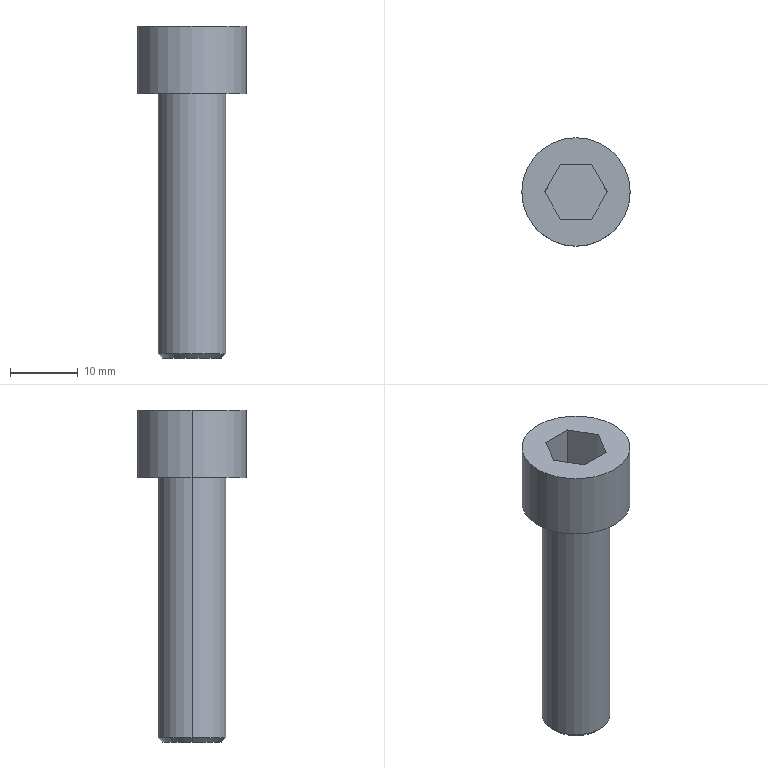Part | Creo | 1 solid | 16 faces | box 16 x 16 x 49 mm | volume 4702 mm3 | plane 10 | cylinder 4 | cone 2 | commonest cylinder face diameters 10 x2 16 x2
STEP:
#1=CARTESIAN_POINT('',(0.,0.,0.));
#2=DIRECTION('',(0.,0.,1.));
#3=DIRECTION('',(1.,0.,0.));
#4=AXIS2_PLACEMENT_3D('',#1,#2,#3);
#5=CARTESIAN_POINT('',(-234.899,34.764,-141.184));
#6=VERTEX_POINT('',#5);
#7=CARTESIAN_POINT('',(-224.899,34.764,-141.184));
#8=VERTEX_POINT('',#7);
#9=CARTESIAN_POINT('',(-229.899,34.764,-141.184));
#10=DIRECTION('',(0.,0.,-1.));
#11=DIRECTION('',(-1.,0.,0.));
#12=AXIS2_PLACEMENT_3D('',#9,#10,#11);
#13=CIRCLE('',#12,5.);
#14=EDGE_CURVE('',#6,#8,#13,.T.);
#15=ORIENTED_EDGE('',*,*,#14,.T.);
#16=CARTESIAN_POINT('',(-224.899,34.764,-102.793));
#17=VERTEX_POINT('',#16);
#18=CARTESIAN_POINT('',(-224.899,34.764,-102.793));
#19=DIRECTION('',(0.,0.,-1.));
#20=VECTOR('',#19,38.391);
#21=LINE('',#18,#20);
#22=EDGE_CURVE('',#17,#8,#21,.T.);
#23=ORIENTED_EDGE('',*,*,#22,.F.);
#24=CARTESIAN_POINT('',(-234.899,34.764,-102.793));
#25=VERTEX_POINT('',#24);
#26=CARTESIAN_POINT('',(-229.899,34.764,-102.793));
#27=DIRECTION('',(0.,0.,1.));
#28=DIRECTION('',(1.,0.,0.));
#29=AXIS2_PLACEMENT_3D('',#26,#27,#28);
#30=CIRCLE('',#29,5.);
#31=EDGE_CURVE('',#17,#25,#30,.T.);
#32=ORIENTED_EDGE('',*,*,#31,.T.);
#33=CARTESIAN_POINT('',(-234.899,34.764,-102.793));
#34=DIRECTION('',(0.,0.,-1.));
#35=VECTOR('',#34,38.391);
#36=LINE('',#33,#35);
#37=EDGE_CURVE('',#25,#6,#36,.T.);
#38=ORIENTED_EDGE('',*,*,#37,.T.);
#39=EDGE_LOOP('',(#15,#23,#32,#38));
#40=FACE_OUTER_BOUND('',#39,.F.);
#41=CARTESIAN_POINT('',(-229.899,34.764,-102.793));
#42=DIRECTION('',(0.,0.,-1.));
#43=DIRECTION('',(-1.,0.,0.));
#44=AXIS2_PLACEMENT_3D('',#41,#42,#43);
#45=CYLINDRICAL_SURFACE('',#44,5.);
#46=ADVANCED_FACE('',(#40),#45,.T.);
#47=CARTESIAN_POINT('',(-234.29,34.764,-141.793));
#48=VERTEX_POINT('',#47);
#49=CARTESIAN_POINT('',(-225.508,34.764,-141.793));
#50=VERTEX_POINT('',#49);
#51=CARTESIAN_POINT('',(-229.899,34.764,-141.793));
#52=DIRECTION('',(0.,0.,-1.));
#53=DIRECTION('',(-1.,0.,0.));
#54=AXIS2_PLACEMENT_3D('',#51,#52,#53);
#55=CIRCLE('',#54,4.391);
#56=EDGE_CURVE('',#48,#50,#55,.T.);
#57=ORIENTED_EDGE('',*,*,#56,.T.);
#58=CARTESIAN_POINT('',(-225.508,34.764,-141.793));
#59=DIRECTION('',(0.7071,0.,0.7071));
#60=VECTOR('',#59,0.8611);
#61=LINE('',#58,#60);
#62=EDGE_CURVE('',#50,#8,#61,.T.);
#63=ORIENTED_EDGE('',*,*,#62,.T.);
#64=ORIENTED_EDGE('',*,*,#14,.F.);
#65=CARTESIAN_POINT('',(-234.29,34.764,-141.793));
#66=DIRECTION('',(-0.7071,0.,0.7071));
#67=VECTOR('',#66,0.8611);
#68=LINE('',#65,#67);
#69=EDGE_CURVE('',#48,#6,#68,.T.);
#70=ORIENTED_EDGE('',*,*,#69,.F.);
#71=EDGE_LOOP('',(#57,#63,#64,#70));
#72=FACE_OUTER_BOUND('',#71,.F.);
#73=CARTESIAN_POINT('',(-229.899,34.764,-141.489));
#74=DIRECTION('',(0.,0.,1.));
#75=DIRECTION('',(1.,0.,0.));
#76=AXIS2_PLACEMENT_3D('',#73,#74,#75);
#77=CONICAL_SURFACE('',#76,4.696,45.);
#78=ADVANCED_FACE('',(#72),#77,.T.);
#79=CARTESIAN_POINT('',(-229.899,34.764,-141.793));
#80=DIRECTION('',(0.,0.,-1.));
#81=DIRECTION('',(1.,0.,0.));
#82=AXIS2_PLACEMENT_3D('',#79,#80,#81);
#83=CIRCLE('',#82,4.391);
#84=EDGE_CURVE('',#50,#48,#83,.T.);
#85=ORIENTED_EDGE('',*,*,#84,.F.);
#86=ORIENTED_EDGE('',*,*,#56,.F.);
#87=EDGE_LOOP('',(#85,#86));
#88=FACE_OUTER_BOUND('',#87,.F.);
#89=CARTESIAN_POINT('',(-229.899,34.764,-141.793));
#90=DIRECTION('',(0.,0.,1.));
#91=DIRECTION('',(1.,0.,0.));
#92=AXIS2_PLACEMENT_3D('',#89,#90,#91);
#93=PLANE('',#92);
#94=ADVANCED_FACE('',(#88),#93,.F.);
#95=ORIENTED_EDGE('',*,*,#84,.T.);
#96=ORIENTED_EDGE('',*,*,#69,.T.);
#97=CARTESIAN_POINT('',(-229.899,34.764,-141.184));
#98=DIRECTION('',(0.,0.,-1.));
#99=DIRECTION('',(1.,0.,0.));
#100=AXIS2_PLACEMENT_3D('',#97,#98,#99);
#101=CIRCLE('',#100,5.);
#102=EDGE_CURVE('',#8,#6,#101,.T.);
#103=ORIENTED_EDGE('',*,*,#102,.F.);
#104=ORIENTED_EDGE('',*,*,#62,.F.);
#105=EDGE_LOOP('',(#95,#96,#103,#104));
#106=FACE_OUTER_BOUND('',#105,.F.);
#107=CARTESIAN_POINT('',(-229.899,34.764,-141.489));
#108=DIRECTION('',(0.,0.,1.));
#109=DIRECTION('',(1.,0.,0.));
#110=AXIS2_PLACEMENT_3D('',#107,#108,#109);
#111=CONICAL_SURFACE('',#110,4.696,45.);
#112=ADVANCED_FACE('',(#106),#111,.T.);
#113=ORIENTED_EDGE('',*,*,#102,.T.);
#114=ORIENTED_EDGE('',*,*,#37,.F.);
#115=CARTESIAN_POINT('',(-229.899,34.764,-102.793));
#116=DIRECTION('',(0.,0.,1.));
#117=DIRECTION('',(-1.,0.,0.));
#118=AXIS2_PLACEMENT_3D('',#115,#116,#117);
#119=CIRCLE('',#118,5.);
#120=EDGE_CURVE('',#25,#17,#119,.T.);
#121=ORIENTED_EDGE('',*,*,#120,.T.);
#122=ORIENTED_EDGE('',*,*,#22,.T.);
#123=EDGE_LOOP('',(#113,#114,#121,#122));
#124=FACE_OUTER_BOUND('',#123,.F.);
#125=CARTESIAN_POINT('',(-229.899,34.764,-102.793));
#126=DIRECTION('',(0.,0.,-1.));
#127=DIRECTION('',(-1.,0.,0.));
#128=AXIS2_PLACEMENT_3D('',#125,#126,#127);
#129=CYLINDRICAL_SURFACE('',#128,5.);
#130=ADVANCED_FACE('',(#124),#129,.T.);
#131=CARTESIAN_POINT('',(-221.899,34.764,-102.793));
#132=VERTEX_POINT('',#131);
#133=CARTESIAN_POINT('',(-237.899,34.764,-102.793));
#134=VERTEX_POINT('',#133);
#135=CARTESIAN_POINT('',(-229.899,34.764,-102.793));
#136=DIRECTION('',(0.,0.,-1.));
#137=DIRECTION('',(1.,0.,0.));
#138=AXIS2_PLACEMENT_3D('',#135,#136,#137);
#139=CIRCLE('',#138,8.);
#140=EDGE_CURVE('',#132,#134,#139,.T.);
#141=ORIENTED_EDGE('',*,*,#140,.F.);
#142=CARTESIAN_POINT('',(-229.899,34.764,-102.793));
#143=DIRECTION('',(0.,0.,-1.));
#144=DIRECTION('',(-1.,0.,0.));
#145=AXIS2_PLACEMENT_3D('',#142,#143,#144);
#146=CIRCLE('',#145,8.);
#147=EDGE_CURVE('',#134,#132,#146,.T.);
#148=ORIENTED_EDGE('',*,*,#147,.F.);
#149=EDGE_LOOP('',(#141,#148));
#150=FACE_OUTER_BOUND('',#149,.F.);
#151=ORIENTED_EDGE('',*,*,#31,.F.);
#152=ORIENTED_EDGE('',*,*,#120,.F.);
#153=EDGE_LOOP('',(#151,#152));
#154=FACE_BOUND('',#153,.F.);
#155=CARTESIAN_POINT('',(-229.899,34.764,-102.793));
#156=DIRECTION('',(0.,0.,-1.));
#157=DIRECTION('',(-1.,0.,0.));
#158=AXIS2_PLACEMENT_3D('',#155,#156,#157);
#159=PLANE('',#158);
#160=ADVANCED_FACE('',(#150,#154),#159,.T.);
#161=CARTESIAN_POINT('',(-237.899,34.764,-92.793));
#162=VERTEX_POINT('',#161);
#163=CARTESIAN_POINT('',(-221.899,34.764,-92.793));
#164=VERTEX_POINT('',#163);
#165=CARTESIAN_POINT('',(-229.899,34.764,-92.793));
#166=DIRECTION('',(0.,0.,1.));
#167=DIRECTION('',(-1.,0.,0.));
#168=AXIS2_PLACEMENT_3D('',#165,#166,#167);
#169=CIRCLE('',#168,8.);
#170=EDGE_CURVE('',#162,#164,#169,.T.);
#171=ORIENTED_EDGE('',*,*,#170,.T.);
#172=CARTESIAN_POINT('',(-221.899,34.764,-102.793));
#173=DIRECTION('',(0.,0.,1.));
#174=VECTOR('',#173,10.);
#175=LINE('',#172,#174);
#176=EDGE_CURVE('',#132,#164,#175,.T.);
#177=ORIENTED_EDGE('',*,*,#176,.F.);
#178=ORIENTED_EDGE('',*,*,#140,.T.);
#179=CARTESIAN_POINT('',(-237.899,34.764,-102.793));
#180=DIRECTION('',(0.,0.,1.));
#181=VECTOR('',#180,10.);
#182=LINE('',#179,#181);
#183=EDGE_CURVE('',#134,#162,#182,.T.);
#184=ORIENTED_EDGE('',*,*,#183,.T.);
#185=EDGE_LOOP('',(#171,#177,#178,#184));
#186=FACE_OUTER_BOUND('',#185,.F.);
#187=CARTESIAN_POINT('',(-229.899,34.764,-102.793));
#188=DIRECTION('',(0.,0.,1.));
#189=DIRECTION('',(1.,0.,0.));
#190=AXIS2_PLACEMENT_3D('',#187,#188,#189);
#191=CYLINDRICAL_SURFACE('',#190,8.);
#192=ADVANCED_FACE('',(#186),#191,.T.);
#193=CARTESIAN_POINT('',(-229.899,34.764,-92.793));
#194=DIRECTION('',(0.,0.,1.));
#195=DIRECTION('',(1.,0.,0.));
#196=AXIS2_PLACEMENT_3D('',#193,#194,#195);
#197=CIRCLE('',#196,8.);
#198=EDGE_CURVE('',#164,#162,#197,.T.);
#199=ORIENTED_EDGE('',*,*,#198,.F.);
#200=ORIENTED_EDGE('',*,*,#170,.F.);
#201=EDGE_LOOP('',(#199,#200));
#202=FACE_OUTER_BOUND('',#201,.F.);
#203=CARTESIAN_POINT('',(-227.59,30.764,-92.793));
#204=VERTEX_POINT('',#203);
#205=CARTESIAN_POINT('',(-232.209,30.764,-92.793));
#206=VERTEX_POINT('',#205);
#207=CARTESIAN_POINT('',(-227.59,30.764,-92.793));
#208=DIRECTION('',(-1.,0.,0.));
#209=VECTOR('',#208,4.619);
#210=LINE('',#207,#209);
#211=EDGE_CURVE('',#204,#206,#210,.T.);
#212=ORIENTED_EDGE('',*,*,#211,.F.);
#213=CARTESIAN_POINT('',(-225.28,34.764,-92.793));
#214=VERTEX_POINT('',#213);
#215=CARTESIAN_POINT('',(-225.28,34.764,-92.793));
#216=DIRECTION('',(-0.5,-0.866,0.));
#217=VECTOR('',#216,4.619);
#218=LINE('',#215,#217);
#219=EDGE_CURVE('',#214,#204,#218,.T.);
#220=ORIENTED_EDGE('',*,*,#219,.F.);
#221=CARTESIAN_POINT('',(-227.59,38.764,-92.793));
#222=VERTEX_POINT('',#221);
#223=CARTESIAN_POINT('',(-227.59,38.764,-92.793));
#224=DIRECTION('',(0.5,-0.866,0.));
#225=VECTOR('',#224,4.619);
#226=LINE('',#223,#225);
#227=EDGE_CURVE('',#222,#214,#226,.T.);
#228=ORIENTED_EDGE('',*,*,#227,.F.);
#229=CARTESIAN_POINT('',(-232.209,38.764,-92.793));
#230=VERTEX_POINT('',#229);
#231=CARTESIAN_POINT('',(-232.209,38.764,-92.793));
#232=DIRECTION('',(1.,0.,0.));
#233=VECTOR('',#232,4.619);
#234=LINE('',#231,#233);
#235=EDGE_CURVE('',#230,#222,#234,.T.);
#236=ORIENTED_EDGE('',*,*,#235,.F.);
#237=CARTESIAN_POINT('',(-234.518,34.764,-92.793));
#238=VERTEX_POINT('',#237);
#239=CARTESIAN_POINT('',(-234.518,34.764,-92.793));
#240=DIRECTION('',(0.5,0.866,0.));
#241=VECTOR('',#240,4.619);
#242=LINE('',#239,#241);
#243=EDGE_CURVE('',#238,#230,#242,.T.);
#244=ORIENTED_EDGE('',*,*,#243,.F.);
#245=CARTESIAN_POINT('',(-232.209,30.764,-92.793));
#246=DIRECTION('',(-0.5,0.866,0.));
#247=VECTOR('',#246,4.619);
#248=LINE('',#245,#247);
#249=EDGE_CURVE('',#206,#238,#248,.T.);
#250=ORIENTED_EDGE('',*,*,#249,.F.);
#251=EDGE_LOOP('',(#212,#220,#228,#236,#244,#250));
#252=FACE_BOUND('',#251,.F.);
#253=CARTESIAN_POINT('',(-229.899,34.764,-92.793));
#254=DIRECTION('',(0.,0.,1.));
#255=DIRECTION('',(1.,0.,0.));
#256=AXIS2_PLACEMENT_3D('',#253,#254,#255);
#257=PLANE('',#256);
#258=ADVANCED_FACE('',(#202,#252),#257,.T.);
#259=ORIENTED_EDGE('',*,*,#211,.T.);
#260=CARTESIAN_POINT('',(-232.209,30.764,-99.393));
#261=VERTEX_POINT('',#260);
#262=CARTESIAN_POINT('',(-232.209,30.764,-92.793));
#263=DIRECTION('',(0.,0.,-1.));
#264=VECTOR('',#263,6.6);
#265=LINE('',#262,#264);
#266=EDGE_CURVE('',#206,#261,#265,.T.);
#267=ORIENTED_EDGE('',*,*,#266,.T.);
#268=CARTESIAN_POINT('',(-227.59,30.764,-99.393));
#269=VERTEX_POINT('',#268);
#270=CARTESIAN_POINT('',(-227.59,30.764,-99.393));
#271=DIRECTION('',(-1.,0.,0.));
#272=VECTOR('',#271,4.619);
#273=LINE('',#270,#272);
#274=EDGE_CURVE('',#269,#261,#273,.T.);
#275=ORIENTED_EDGE('',*,*,#274,.F.);
#276=CARTESIAN_POINT('',(-227.59,30.764,-92.793));
#277=DIRECTION('',(0.,0.,-1.));
#278=VECTOR('',#277,6.6);
#279=LINE('',#276,#278);
#280=EDGE_CURVE('',#204,#269,#279,.T.);
#281=ORIENTED_EDGE('',*,*,#280,.F.);
#282=EDGE_LOOP('',(#259,#267,#275,#281));
#283=FACE_OUTER_BOUND('',#282,.F.);
#284=CARTESIAN_POINT('',(-232.209,30.764,-99.393));
#285=DIRECTION('',(0.,-1.,0.));
#286=DIRECTION('',(0.,0.,-1.));
#287=AXIS2_PLACEMENT_3D('',#284,#285,#286);
#288=PLANE('',#287);
#289=ADVANCED_FACE('',(#283),#288,.F.);
#290=ORIENTED_EDGE('',*,*,#249,.T.);
#291=CARTESIAN_POINT('',(-234.518,34.764,-99.393));
#292=VERTEX_POINT('',#291);
#293=CARTESIAN_POINT('',(-234.518,34.764,-92.793));
#294=DIRECTION('',(0.,0.,-1.));
#295=VECTOR('',#294,6.6);
#296=LINE('',#293,#295);
#297=EDGE_CURVE('',#238,#292,#296,.T.);
#298=ORIENTED_EDGE('',*,*,#297,.T.);
#299=CARTESIAN_POINT('',(-234.518,34.764,-99.393));
#300=DIRECTION('',(0.5,-0.866,0.));
#301=VECTOR('',#300,4.619);
#302=LINE('',#299,#301);
#303=EDGE_CURVE('',#292,#261,#302,.T.);
#304=ORIENTED_EDGE('',*,*,#303,.T.);
#305=ORIENTED_EDGE('',*,*,#266,.F.);
#306=EDGE_LOOP('',(#290,#298,#304,#305));
#307=FACE_OUTER_BOUND('',#306,.F.);
#308=CARTESIAN_POINT('',(-234.518,34.764,-99.393));
#309=DIRECTION('',(-0.866,-0.5,0.));
#310=DIRECTION('',(0.5,-0.866,0.));
#311=AXIS2_PLACEMENT_3D('',#308,#309,#310);
#312=PLANE('',#311);
#313=ADVANCED_FACE('',(#307),#312,.F.);
#314=ORIENTED_EDGE('',*,*,#243,.T.);
#315=CARTESIAN_POINT('',(-232.209,38.764,-99.393));
#316=VERTEX_POINT('',#315);
#317=CARTESIAN_POINT('',(-232.209,38.764,-92.793));
#318=DIRECTION('',(0.,0.,-1.));
#319=VECTOR('',#318,6.6);
#320=LINE('',#317,#319);
#321=EDGE_CURVE('',#230,#316,#320,.T.);
#322=ORIENTED_EDGE('',*,*,#321,.T.);
#323=CARTESIAN_POINT('',(-232.209,38.764,-99.393));
#324=DIRECTION('',(-0.5,-0.866,0.));
#325=VECTOR('',#324,4.619);
#326=LINE('',#323,#325);
#327=EDGE_CURVE('',#316,#292,#326,.T.);
#328=ORIENTED_EDGE('',*,*,#327,.T.);
#329=ORIENTED_EDGE('',*,*,#297,.F.);
#330=EDGE_LOOP('',(#314,#322,#328,#329));
#331=FACE_OUTER_BOUND('',#330,.F.);
#332=CARTESIAN_POINT('',(-232.209,38.764,-99.393));
#333=DIRECTION('',(-0.866,0.5,0.));
#334=DIRECTION('',(-0.5,-0.866,0.));
#335=AXIS2_PLACEMENT_3D('',#332,#333,#334);
#336=PLANE('',#335);
#337=ADVANCED_FACE('',(#331),#336,.F.);
#338=ORIENTED_EDGE('',*,*,#235,.T.);
#339=CARTESIAN_POINT('',(-227.59,38.764,-99.393));
#340=VERTEX_POINT('',#339);
#341=CARTESIAN_POINT('',(-227.59,38.764,-92.793));
#342=DIRECTION('',(0.,0.,-1.));
#343=VECTOR('',#342,6.6);
#344=LINE('',#341,#343);
#345=EDGE_CURVE('',#222,#340,#344,.T.);
#346=ORIENTED_EDGE('',*,*,#345,.T.);
#347=CARTESIAN_POINT('',(-232.209,38.764,-99.393));
#348=DIRECTION('',(1.,0.,0.));
#349=VECTOR('',#348,4.619);
#350=LINE('',#347,#349);
#351=EDGE_CURVE('',#316,#340,#350,.T.);
#352=ORIENTED_EDGE('',*,*,#351,.F.);
#353=ORIENTED_EDGE('',*,*,#321,.F.);
#354=EDGE_LOOP('',(#338,#346,#352,#353));
#355=FACE_OUTER_BOUND('',#354,.F.);
#356=CARTESIAN_POINT('',(-227.59,38.764,-99.393));
#357=DIRECTION('',(0.,1.,0.));
#358=DIRECTION('',(0.,0.,1.));
#359=AXIS2_PLACEMENT_3D('',#356,#357,#358);
#360=PLANE('',#359);
#361=ADVANCED_FACE('',(#355),#360,.F.);
#362=ORIENTED_EDGE('',*,*,#227,.T.);
#363=CARTESIAN_POINT('',(-225.28,34.764,-99.393));
#364=VERTEX_POINT('',#363);
#365=CARTESIAN_POINT('',(-225.28,34.764,-92.793));
#366=DIRECTION('',(0.,0.,-1.));
#367=VECTOR('',#366,6.6);
#368=LINE('',#365,#367);
#369=EDGE_CURVE('',#214,#364,#368,.T.);
#370=ORIENTED_EDGE('',*,*,#369,.T.);
#371=CARTESIAN_POINT('',(-225.28,34.764,-99.393));
#372=DIRECTION('',(-0.5,0.866,0.));
#373=VECTOR('',#372,4.619);
#374=LINE('',#371,#373);
#375=EDGE_CURVE('',#364,#340,#374,.T.);
#376=ORIENTED_EDGE('',*,*,#375,.T.);
#377=ORIENTED_EDGE('',*,*,#345,.F.);
#378=EDGE_LOOP('',(#362,#370,#376,#377));
#379=FACE_OUTER_BOUND('',#378,.F.);
#380=CARTESIAN_POINT('',(-225.28,34.764,-99.393));
#381=DIRECTION('',(0.866,0.5,0.));
#382=DIRECTION('',(-0.5,0.866,0.));
#383=AXIS2_PLACEMENT_3D('',#380,#381,#382);
#384=PLANE('',#383);
#385=ADVANCED_FACE('',(#379),#384,.F.);
#386=ORIENTED_EDGE('',*,*,#219,.T.);
#387=ORIENTED_EDGE('',*,*,#280,.T.);
#388=CARTESIAN_POINT('',(-227.59,30.764,-99.393));
#389=DIRECTION('',(0.5,0.866,0.));
#390=VECTOR('',#389,4.619);
#391=LINE('',#388,#390);
#392=EDGE_CURVE('',#269,#364,#391,.T.);
#393=ORIENTED_EDGE('',*,*,#392,.T.);
#394=ORIENTED_EDGE('',*,*,#369,.F.);
#395=EDGE_LOOP('',(#386,#387,#393,#394));
#396=FACE_OUTER_BOUND('',#395,.F.);
#397=CARTESIAN_POINT('',(-227.59,30.764,-99.393));
#398=DIRECTION('',(0.866,-0.5,0.));
#399=DIRECTION('',(0.5,0.866,0.));
#400=AXIS2_PLACEMENT_3D('',#397,#398,#399);
#401=PLANE('',#400);
#402=ADVANCED_FACE('',(#396),#401,.F.);
#403=ORIENTED_EDGE('',*,*,#274,.T.);
#404=ORIENTED_EDGE('',*,*,#303,.F.);
#405=ORIENTED_EDGE('',*,*,#327,.F.);
#406=ORIENTED_EDGE('',*,*,#351,.T.);
#407=ORIENTED_EDGE('',*,*,#375,.F.);
#408=ORIENTED_EDGE('',*,*,#392,.F.);
#409=EDGE_LOOP('',(#403,#404,#405,#406,#407,#408));
#410=FACE_OUTER_BOUND('',#409,.F.);
#411=CARTESIAN_POINT('',(-227.59,30.764,-99.393));
#412=DIRECTION('',(0.,0.,1.));
#413=DIRECTION('',(1.,0.,0.));
#414=AXIS2_PLACEMENT_3D('',#411,#412,#413);
#415=PLANE('',#414);
#416=ADVANCED_FACE('',(#410),#415,.T.);
#417=ORIENTED_EDGE('',*,*,#198,.T.);
#418=ORIENTED_EDGE('',*,*,#183,.F.);
#419=ORIENTED_EDGE('',*,*,#147,.T.);
#420=ORIENTED_EDGE('',*,*,#176,.T.);
#421=EDGE_LOOP('',(#417,#418,#419,#420));
#422=FACE_OUTER_BOUND('',#421,.F.);
#423=CARTESIAN_POINT('',(-229.899,34.764,-102.793));
#424=DIRECTION('',(0.,0.,1.));
#425=DIRECTION('',(1.,0.,0.));
#426=AXIS2_PLACEMENT_3D('',#423,#424,#425);
#427=CYLINDRICAL_SURFACE('',#426,8.);
#428=ADVANCED_FACE('',(#422),#427,.T.);
#429=CLOSED_SHELL('',(#46,#78,#94,#112,#130,#160,#192,#258,#289,#313,#337,#361,#385,#402,#416,#428));
#430=MANIFOLD_SOLID_BREP('',#429);
#431=(LENGTH_UNIT()NAMED_UNIT(*)SI_UNIT(.MILLI.,.METRE.));
#432=UNCERTAINTY_MEASURE_WITH_UNIT(LENGTH_MEASURE(0.005397),#431,'','');
#433=(NAMED_UNIT(*)PLANE_ANGLE_UNIT()SI_UNIT($,.RADIAN.));
#434=PLANE_ANGLE_MEASURE_WITH_UNIT(PLANE_ANGLE_MEASURE(0.01745),#433);
#435=(CONVERSION_BASED_UNIT('DEGREE',#434)NAMED_UNIT(*)PLANE_ANGLE_UNIT());
#436=(NAMED_UNIT(*)SI_UNIT($,.STERADIAN.)SOLID_ANGLE_UNIT());
#437=(GEOMETRIC_REPRESENTATION_CONTEXT(3)GLOBAL_UNCERTAINTY_ASSIGNED_CONTEXT((#432))GLOBAL_UNIT_ASSIGNED_CONTEXT((#431,#435,#436))REPRESENTATION_CONTEXT('',''));
#438=ADVANCED_BREP_SHAPE_REPRESENTATION('',(#4,#430),#437);